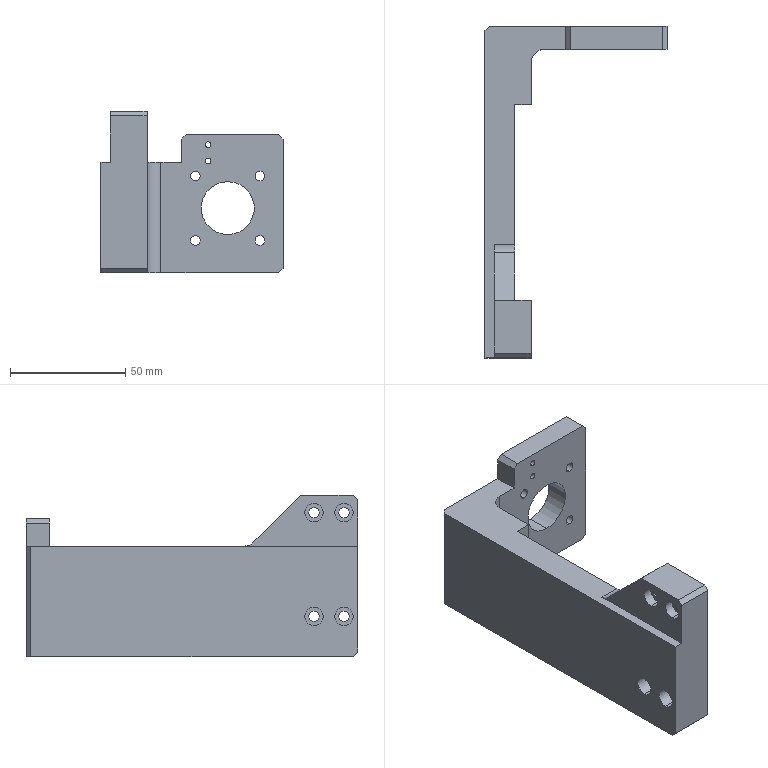Part | SolidWorks | features ICE 5, Chamfer 3, HoleWzd 3, Fillet 2, Extrusion 1 | 1 solid | 59 faces | box 79 x 144 x 70 mm | volume 147629 mm3 | cylinder 32 | plane 27 | commonest cylinder face diameters 4.2 x8 4.5 x8 8 x8 2.5 x4 23 x2 10 x1